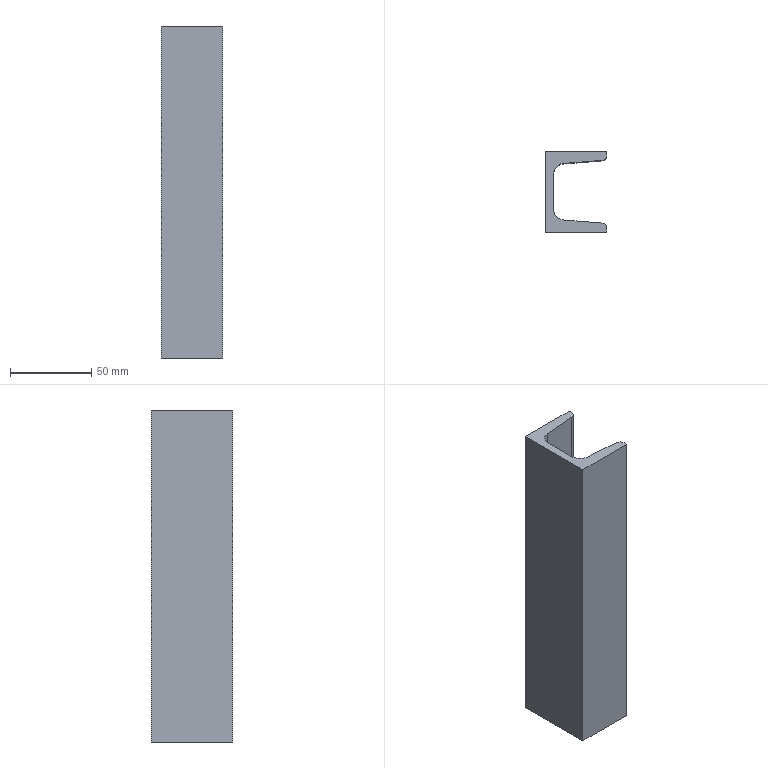Part | STEP file | DIN 1026-1 U 50 1785357045599 | 1 solid | 14 faces | box 38 x 50 x 204.153 mm | volume 145329 mm3 | plane 10 | cylinder 4 | commonest cylinder face diameters 7 x2 14 x2
STEP:
#1=CARTESIAN_POINT('',(5.,-10.418,254.153));
#2=VERTEX_POINT('',#1);
#3=CARTESIAN_POINT('',(11.442,-17.395,254.153));
#4=VERTEX_POINT('',#3);
#5=CARTESIAN_POINT('',(12.,-10.418,254.153));
#6=DIRECTION('',(0.,0.,1.));
#7=DIRECTION('',(-1.,0.,0.));
#8=AXIS2_PLACEMENT_3D('',#5,#6,#7);
#9=CIRCLE('',#8,7.);
#10=EDGE_CURVE('',#2,#4,#9,.T.);
#11=ORIENTED_EDGE('',*,*,#10,.T.);
#12=CARTESIAN_POINT('',(11.442,-17.395,50.));
#13=VERTEX_POINT('',#12);
#14=CARTESIAN_POINT('',(11.442,-17.395,0.));
#15=DIRECTION('',(0.,0.,1.));
#16=VECTOR('',#15,10.);
#17=LINE('',#14,#16);
#18=EDGE_CURVE('',#13,#4,#17,.T.);
#19=ORIENTED_EDGE('',*,*,#18,.F.);
#20=CARTESIAN_POINT('',(5.,-10.418,50.));
#21=VERTEX_POINT('',#20);
#22=CARTESIAN_POINT('',(12.,-10.418,50.));
#23=DIRECTION('',(0.,0.,1.));
#24=DIRECTION('',(-1.,0.,0.));
#25=AXIS2_PLACEMENT_3D('',#22,#23,#24);
#26=CIRCLE('',#25,7.);
#27=EDGE_CURVE('',#21,#13,#26,.T.);
#28=ORIENTED_EDGE('',*,*,#27,.F.);
#29=CARTESIAN_POINT('',(5.,-10.418,0.));
#30=DIRECTION('',(0.,0.,1.));
#31=VECTOR('',#30,10.);
#32=LINE('',#29,#31);
#33=EDGE_CURVE('',#21,#2,#32,.T.);
#34=ORIENTED_EDGE('',*,*,#33,.T.);
#35=EDGE_LOOP('',(#11,#19,#28,#34));
#36=FACE_OUTER_BOUND('',#35,.T.);
#37=CARTESIAN_POINT('',(12.,-10.418,0.));
#38=DIRECTION('',(0.,0.,1.));
#39=DIRECTION('',(-1.,0.,0.));
#40=AXIS2_PLACEMENT_3D('',#37,#38,#39);
#41=CYLINDRICAL_SURFACE('',#40,7.);
#42=ADVANCED_FACE('',(#36),#41,.F.);
#43=CARTESIAN_POINT('',(34.779,-19.262,254.153));
#44=VERTEX_POINT('',#43);
#45=CARTESIAN_POINT('',(14.505,-17.64,254.153));
#46=DIRECTION('',(0.9968,-0.07975,0.));
#47=VECTOR('',#46,10.);
#48=LINE('',#45,#47);
#49=EDGE_CURVE('',#4,#44,#48,.T.);
#50=ORIENTED_EDGE('',*,*,#49,.T.);
#51=CARTESIAN_POINT('',(34.779,-19.262,50.));
#52=VERTEX_POINT('',#51);
#53=CARTESIAN_POINT('',(34.779,-19.262,0.));
#54=DIRECTION('',(0.,0.,1.));
#55=VECTOR('',#54,10.);
#56=LINE('',#53,#55);
#57=EDGE_CURVE('',#52,#44,#56,.T.);
#58=ORIENTED_EDGE('',*,*,#57,.F.);
#59=CARTESIAN_POINT('',(14.505,-17.64,50.));
#60=DIRECTION('',(0.9968,-0.07975,0.));
#61=VECTOR('',#60,10.);
#62=LINE('',#59,#61);
#63=EDGE_CURVE('',#13,#52,#62,.T.);
#64=ORIENTED_EDGE('',*,*,#63,.F.);
#65=ORIENTED_EDGE('',*,*,#18,.T.);
#66=EDGE_LOOP('',(#50,#58,#64,#65));
#67=FACE_OUTER_BOUND('',#66,.T.);
#68=CARTESIAN_POINT('',(11.442,-17.395,0.));
#69=DIRECTION('',(0.07975,0.9968,0.));
#70=DIRECTION('',(0.,0.,1.));
#71=AXIS2_PLACEMENT_3D('',#68,#69,#70);
#72=PLANE('',#71);
#73=ADVANCED_FACE('',(#67),#72,.T.);
#74=CARTESIAN_POINT('',(38.,-22.751,254.153));
#75=VERTEX_POINT('',#74);
#76=CARTESIAN_POINT('',(34.5,-22.751,254.153));
#77=DIRECTION('',(0.,0.,-1.));
#78=DIRECTION('',(-1.,0.,0.));
#79=AXIS2_PLACEMENT_3D('',#76,#77,#78);
#80=CIRCLE('',#79,3.5);
#81=EDGE_CURVE('',#44,#75,#80,.T.);
#82=ORIENTED_EDGE('',*,*,#81,.T.);
#83=CARTESIAN_POINT('',(38.,-22.751,50.));
#84=VERTEX_POINT('',#83);
#85=CARTESIAN_POINT('',(38.,-22.751,0.));
#86=DIRECTION('',(0.,0.,1.));
#87=VECTOR('',#86,10.);
#88=LINE('',#85,#87);
#89=EDGE_CURVE('',#84,#75,#88,.T.);
#90=ORIENTED_EDGE('',*,*,#89,.F.);
#91=CARTESIAN_POINT('',(34.5,-22.751,50.));
#92=DIRECTION('',(0.,0.,-1.));
#93=DIRECTION('',(-1.,0.,0.));
#94=AXIS2_PLACEMENT_3D('',#91,#92,#93);
#95=CIRCLE('',#94,3.5);
#96=EDGE_CURVE('',#52,#84,#95,.T.);
#97=ORIENTED_EDGE('',*,*,#96,.F.);
#98=ORIENTED_EDGE('',*,*,#57,.T.);
#99=EDGE_LOOP('',(#82,#90,#97,#98));
#100=FACE_OUTER_BOUND('',#99,.T.);
#101=CARTESIAN_POINT('',(34.5,-22.751,0.));
#102=DIRECTION('',(0.,0.,1.));
#103=DIRECTION('',(-1.,0.,0.));
#104=AXIS2_PLACEMENT_3D('',#101,#102,#103);
#105=CYLINDRICAL_SURFACE('',#104,3.5);
#106=ADVANCED_FACE('',(#100),#105,.T.);
#107=CARTESIAN_POINT('',(38.,-25.,254.153));
#108=VERTEX_POINT('',#107);
#109=CARTESIAN_POINT('',(38.,-11.376,254.153));
#110=DIRECTION('',(0.,-1.,0.));
#111=VECTOR('',#110,10.);
#112=LINE('',#109,#111);
#113=EDGE_CURVE('',#75,#108,#112,.T.);
#114=ORIENTED_EDGE('',*,*,#113,.T.);
#115=CARTESIAN_POINT('',(38.,-25.,50.));
#116=VERTEX_POINT('',#115);
#117=CARTESIAN_POINT('',(38.,-25.,0.));
#118=DIRECTION('',(0.,0.,1.));
#119=VECTOR('',#118,10.);
#120=LINE('',#117,#119);
#121=EDGE_CURVE('',#116,#108,#120,.T.);
#122=ORIENTED_EDGE('',*,*,#121,.F.);
#123=CARTESIAN_POINT('',(38.,-11.376,50.));
#124=DIRECTION('',(0.,-1.,0.));
#125=VECTOR('',#124,10.);
#126=LINE('',#123,#125);
#127=EDGE_CURVE('',#84,#116,#126,.T.);
#128=ORIENTED_EDGE('',*,*,#127,.F.);
#129=ORIENTED_EDGE('',*,*,#89,.T.);
#130=EDGE_LOOP('',(#114,#122,#128,#129));
#131=FACE_OUTER_BOUND('',#130,.T.);
#132=CARTESIAN_POINT('',(38.,-22.751,0.));
#133=DIRECTION('',(1.,0.,0.));
#134=DIRECTION('',(0.,0.,-1.));
#135=AXIS2_PLACEMENT_3D('',#132,#133,#134);
#136=PLANE('',#135);
#137=ADVANCED_FACE('',(#131),#136,.T.);
#138=CARTESIAN_POINT('',(0.,-25.,254.153));
#139=VERTEX_POINT('',#138);
#140=CARTESIAN_POINT('',(28.5,-25.,254.153));
#141=DIRECTION('',(-1.,0.,0.));
#142=VECTOR('',#141,10.);
#143=LINE('',#140,#142);
#144=EDGE_CURVE('',#108,#139,#143,.T.);
#145=ORIENTED_EDGE('',*,*,#144,.T.);
#146=CARTESIAN_POINT('',(0.,-25.,50.));
#147=VERTEX_POINT('',#146);
#148=CARTESIAN_POINT('',(0.,-25.,0.));
#149=DIRECTION('',(0.,0.,1.));
#150=VECTOR('',#149,10.);
#151=LINE('',#148,#150);
#152=EDGE_CURVE('',#147,#139,#151,.T.);
#153=ORIENTED_EDGE('',*,*,#152,.F.);
#154=CARTESIAN_POINT('',(28.5,-25.,50.));
#155=DIRECTION('',(-1.,0.,0.));
#156=VECTOR('',#155,10.);
#157=LINE('',#154,#156);
#158=EDGE_CURVE('',#116,#147,#157,.T.);
#159=ORIENTED_EDGE('',*,*,#158,.F.);
#160=ORIENTED_EDGE('',*,*,#121,.T.);
#161=EDGE_LOOP('',(#145,#153,#159,#160));
#162=FACE_OUTER_BOUND('',#161,.T.);
#163=CARTESIAN_POINT('',(38.,-25.,0.));
#164=DIRECTION('',(0.,-1.,0.));
#165=DIRECTION('',(0.,0.,-1.));
#166=AXIS2_PLACEMENT_3D('',#163,#164,#165);
#167=PLANE('',#166);
#168=ADVANCED_FACE('',(#162),#167,.T.);
#169=CARTESIAN_POINT('',(0.,25.,254.153));
#170=VERTEX_POINT('',#169);
#171=CARTESIAN_POINT('',(0.,0.,254.153));
#172=DIRECTION('',(0.,1.,0.));
#173=VECTOR('',#172,10.);
#174=LINE('',#171,#173);
#175=EDGE_CURVE('',#139,#170,#174,.T.);
#176=ORIENTED_EDGE('',*,*,#175,.T.);
#177=CARTESIAN_POINT('',(0.,25.,50.));
#178=VERTEX_POINT('',#177);
#179=CARTESIAN_POINT('',(0.,25.,0.));
#180=DIRECTION('',(0.,0.,1.));
#181=VECTOR('',#180,10.);
#182=LINE('',#179,#181);
#183=EDGE_CURVE('',#178,#170,#182,.T.);
#184=ORIENTED_EDGE('',*,*,#183,.F.);
#185=CARTESIAN_POINT('',(0.,0.,50.));
#186=DIRECTION('',(0.,1.,0.));
#187=VECTOR('',#186,10.);
#188=LINE('',#185,#187);
#189=EDGE_CURVE('',#147,#178,#188,.T.);
#190=ORIENTED_EDGE('',*,*,#189,.F.);
#191=ORIENTED_EDGE('',*,*,#152,.T.);
#192=EDGE_LOOP('',(#176,#184,#190,#191));
#193=FACE_OUTER_BOUND('',#192,.T.);
#194=CARTESIAN_POINT('',(0.,0.,0.));
#195=DIRECTION('',(-1.,0.,0.));
#196=DIRECTION('',(0.,0.,1.));
#197=AXIS2_PLACEMENT_3D('',#194,#195,#196);
#198=PLANE('',#197);
#199=ADVANCED_FACE('',(#193),#198,.T.);
#200=CARTESIAN_POINT('',(38.,25.,254.153));
#201=VERTEX_POINT('',#200);
#202=CARTESIAN_POINT('',(9.5,25.,254.153));
#203=DIRECTION('',(1.,0.,0.));
#204=VECTOR('',#203,10.);
#205=LINE('',#202,#204);
#206=EDGE_CURVE('',#170,#201,#205,.T.);
#207=ORIENTED_EDGE('',*,*,#206,.T.);
#208=CARTESIAN_POINT('',(38.,25.,50.));
#209=VERTEX_POINT('',#208);
#210=CARTESIAN_POINT('',(38.,25.,0.));
#211=DIRECTION('',(0.,0.,1.));
#212=VECTOR('',#211,10.);
#213=LINE('',#210,#212);
#214=EDGE_CURVE('',#209,#201,#213,.T.);
#215=ORIENTED_EDGE('',*,*,#214,.F.);
#216=CARTESIAN_POINT('',(9.5,25.,50.));
#217=DIRECTION('',(1.,0.,0.));
#218=VECTOR('',#217,10.);
#219=LINE('',#216,#218);
#220=EDGE_CURVE('',#178,#209,#219,.T.);
#221=ORIENTED_EDGE('',*,*,#220,.F.);
#222=ORIENTED_EDGE('',*,*,#183,.T.);
#223=EDGE_LOOP('',(#207,#215,#221,#222));
#224=FACE_OUTER_BOUND('',#223,.T.);
#225=CARTESIAN_POINT('',(0.,25.,0.));
#226=DIRECTION('',(0.,1.,0.));
#227=DIRECTION('',(0.,0.,1.));
#228=AXIS2_PLACEMENT_3D('',#225,#226,#227);
#229=PLANE('',#228);
#230=ADVANCED_FACE('',(#224),#229,.T.);
#231=CARTESIAN_POINT('',(38.,22.751,254.153));
#232=VERTEX_POINT('',#231);
#233=CARTESIAN_POINT('',(38.,12.5,254.153));
#234=DIRECTION('',(0.,-1.,0.));
#235=VECTOR('',#234,10.);
#236=LINE('',#233,#235);
#237=EDGE_CURVE('',#201,#232,#236,.T.);
#238=ORIENTED_EDGE('',*,*,#237,.T.);
#239=CARTESIAN_POINT('',(38.,22.751,50.));
#240=VERTEX_POINT('',#239);
#241=CARTESIAN_POINT('',(38.,22.751,0.));
#242=DIRECTION('',(0.,0.,1.));
#243=VECTOR('',#242,10.);
#244=LINE('',#241,#243);
#245=EDGE_CURVE('',#240,#232,#244,.T.);
#246=ORIENTED_EDGE('',*,*,#245,.F.);
#247=CARTESIAN_POINT('',(38.,12.5,50.));
#248=DIRECTION('',(0.,-1.,0.));
#249=VECTOR('',#248,10.);
#250=LINE('',#247,#249);
#251=EDGE_CURVE('',#209,#240,#250,.T.);
#252=ORIENTED_EDGE('',*,*,#251,.F.);
#253=ORIENTED_EDGE('',*,*,#214,.T.);
#254=EDGE_LOOP('',(#238,#246,#252,#253));
#255=FACE_OUTER_BOUND('',#254,.T.);
#256=CARTESIAN_POINT('',(38.,25.,0.));
#257=DIRECTION('',(1.,0.,0.));
#258=DIRECTION('',(0.,0.,-1.));
#259=AXIS2_PLACEMENT_3D('',#256,#257,#258);
#260=PLANE('',#259);
#261=ADVANCED_FACE('',(#255),#260,.T.);
#262=CARTESIAN_POINT('',(34.779,19.262,254.153));
#263=VERTEX_POINT('',#262);
#264=CARTESIAN_POINT('',(34.5,22.751,254.153));
#265=DIRECTION('',(0.,0.,-1.));
#266=DIRECTION('',(-0.07975,0.9968,0.));
#267=AXIS2_PLACEMENT_3D('',#264,#265,#266);
#268=CIRCLE('',#267,3.5);
#269=EDGE_CURVE('',#232,#263,#268,.T.);
#270=ORIENTED_EDGE('',*,*,#269,.T.);
#271=CARTESIAN_POINT('',(34.779,19.262,50.));
#272=VERTEX_POINT('',#271);
#273=CARTESIAN_POINT('',(34.779,19.262,0.));
#274=DIRECTION('',(0.,0.,1.));
#275=VECTOR('',#274,10.);
#276=LINE('',#273,#275);
#277=EDGE_CURVE('',#272,#263,#276,.T.);
#278=ORIENTED_EDGE('',*,*,#277,.F.);
#279=CARTESIAN_POINT('',(34.5,22.751,50.));
#280=DIRECTION('',(0.,0.,-1.));
#281=DIRECTION('',(-0.07975,0.9968,0.));
#282=AXIS2_PLACEMENT_3D('',#279,#280,#281);
#283=CIRCLE('',#282,3.5);
#284=EDGE_CURVE('',#240,#272,#283,.T.);
#285=ORIENTED_EDGE('',*,*,#284,.F.);
#286=ORIENTED_EDGE('',*,*,#245,.T.);
#287=EDGE_LOOP('',(#270,#278,#285,#286));
#288=FACE_OUTER_BOUND('',#287,.T.);
#289=CARTESIAN_POINT('',(34.5,22.751,0.));
#290=DIRECTION('',(0.,0.,1.));
#291=DIRECTION('',(-0.07975,0.9968,0.));
#292=AXIS2_PLACEMENT_3D('',#289,#290,#291);
#293=CYLINDRICAL_SURFACE('',#292,3.5);
#294=ADVANCED_FACE('',(#288),#293,.T.);
#295=CARTESIAN_POINT('',(11.442,17.395,254.153));
#296=VERTEX_POINT('',#295);
#297=CARTESIAN_POINT('',(26.174,18.574,254.153));
#298=DIRECTION('',(-0.9968,-0.07975,0.));
#299=VECTOR('',#298,10.);
#300=LINE('',#297,#299);
#301=EDGE_CURVE('',#263,#296,#300,.T.);
#302=ORIENTED_EDGE('',*,*,#301,.T.);
#303=CARTESIAN_POINT('',(11.442,17.395,50.));
#304=VERTEX_POINT('',#303);
#305=CARTESIAN_POINT('',(11.442,17.395,0.));
#306=DIRECTION('',(0.,0.,1.));
#307=VECTOR('',#306,10.);
#308=LINE('',#305,#307);
#309=EDGE_CURVE('',#304,#296,#308,.T.);
#310=ORIENTED_EDGE('',*,*,#309,.F.);
#311=CARTESIAN_POINT('',(26.174,18.574,50.));
#312=DIRECTION('',(-0.9968,-0.07975,0.));
#313=VECTOR('',#312,10.);
#314=LINE('',#311,#313);
#315=EDGE_CURVE('',#272,#304,#314,.T.);
#316=ORIENTED_EDGE('',*,*,#315,.F.);
#317=ORIENTED_EDGE('',*,*,#277,.T.);
#318=EDGE_LOOP('',(#302,#310,#316,#317));
#319=FACE_OUTER_BOUND('',#318,.T.);
#320=CARTESIAN_POINT('',(34.779,19.262,0.));
#321=DIRECTION('',(0.07975,-0.9968,0.));
#322=DIRECTION('',(0.,0.,-1.));
#323=AXIS2_PLACEMENT_3D('',#320,#321,#322);
#324=PLANE('',#323);
#325=ADVANCED_FACE('',(#319),#324,.T.);
#326=CARTESIAN_POINT('',(5.,10.418,254.153));
#327=VERTEX_POINT('',#326);
#328=CARTESIAN_POINT('',(12.,10.418,254.153));
#329=DIRECTION('',(0.,0.,1.));
#330=DIRECTION('',(-0.07975,0.9968,0.));
#331=AXIS2_PLACEMENT_3D('',#328,#329,#330);
#332=CIRCLE('',#331,7.);
#333=EDGE_CURVE('',#296,#327,#332,.T.);
#334=ORIENTED_EDGE('',*,*,#333,.T.);
#335=CARTESIAN_POINT('',(5.,10.418,50.));
#336=VERTEX_POINT('',#335);
#337=CARTESIAN_POINT('',(5.,10.418,0.));
#338=DIRECTION('',(0.,0.,1.));
#339=VECTOR('',#338,10.);
#340=LINE('',#337,#339);
#341=EDGE_CURVE('',#336,#327,#340,.T.);
#342=ORIENTED_EDGE('',*,*,#341,.F.);
#343=CARTESIAN_POINT('',(12.,10.418,50.));
#344=DIRECTION('',(0.,0.,1.));
#345=DIRECTION('',(-0.07975,0.9968,0.));
#346=AXIS2_PLACEMENT_3D('',#343,#344,#345);
#347=CIRCLE('',#346,7.);
#348=EDGE_CURVE('',#304,#336,#347,.T.);
#349=ORIENTED_EDGE('',*,*,#348,.F.);
#350=ORIENTED_EDGE('',*,*,#309,.T.);
#351=EDGE_LOOP('',(#334,#342,#349,#350));
#352=FACE_OUTER_BOUND('',#351,.T.);
#353=CARTESIAN_POINT('',(12.,10.418,0.));
#354=DIRECTION('',(0.,0.,1.));
#355=DIRECTION('',(-0.07975,0.9968,0.));
#356=AXIS2_PLACEMENT_3D('',#353,#354,#355);
#357=CYLINDRICAL_SURFACE('',#356,7.);
#358=ADVANCED_FACE('',(#352),#357,.F.);
#359=CARTESIAN_POINT('',(5.,0.,254.153));
#360=DIRECTION('',(0.,-1.,0.));
#361=VECTOR('',#360,10.);
#362=LINE('',#359,#361);
#363=EDGE_CURVE('',#327,#2,#362,.T.);
#364=ORIENTED_EDGE('',*,*,#363,.T.);
#365=ORIENTED_EDGE('',*,*,#33,.F.);
#366=CARTESIAN_POINT('',(5.,0.,50.));
#367=DIRECTION('',(0.,-1.,0.));
#368=VECTOR('',#367,10.);
#369=LINE('',#366,#368);
#370=EDGE_CURVE('',#336,#21,#369,.T.);
#371=ORIENTED_EDGE('',*,*,#370,.F.);
#372=ORIENTED_EDGE('',*,*,#341,.T.);
#373=EDGE_LOOP('',(#364,#365,#371,#372));
#374=FACE_OUTER_BOUND('',#373,.T.);
#375=CARTESIAN_POINT('',(5.,0.,0.));
#376=DIRECTION('',(1.,0.,0.));
#377=DIRECTION('',(0.,0.,-1.));
#378=AXIS2_PLACEMENT_3D('',#375,#376,#377);
#379=PLANE('',#378);
#380=ADVANCED_FACE('',(#374),#379,.T.);
#381=ORIENTED_EDGE('',*,*,#220,.T.);
#382=ORIENTED_EDGE('',*,*,#251,.T.);
#383=ORIENTED_EDGE('',*,*,#284,.T.);
#384=ORIENTED_EDGE('',*,*,#315,.T.);
#385=ORIENTED_EDGE('',*,*,#348,.T.);
#386=ORIENTED_EDGE('',*,*,#370,.T.);
#387=ORIENTED_EDGE('',*,*,#27,.T.);
#388=ORIENTED_EDGE('',*,*,#63,.T.);
#389=ORIENTED_EDGE('',*,*,#96,.T.);
#390=ORIENTED_EDGE('',*,*,#127,.T.);
#391=ORIENTED_EDGE('',*,*,#158,.T.);
#392=ORIENTED_EDGE('',*,*,#189,.T.);
#393=EDGE_LOOP('',(#381,#382,#383,#384,#385,#386,#387,#388,#389,#390,#391,#392));
#394=FACE_OUTER_BOUND('',#393,.T.);
#395=CARTESIAN_POINT('',(19.,0.,50.));
#396=DIRECTION('',(0.,0.,1.));
#397=DIRECTION('',(1.,0.,0.));
#398=AXIS2_PLACEMENT_3D('',#395,#396,#397);
#399=PLANE('',#398);
#400=ADVANCED_FACE('',(#394),#399,.F.);
#401=ORIENTED_EDGE('',*,*,#206,.F.);
#402=ORIENTED_EDGE('',*,*,#175,.F.);
#403=ORIENTED_EDGE('',*,*,#144,.F.);
#404=ORIENTED_EDGE('',*,*,#113,.F.);
#405=ORIENTED_EDGE('',*,*,#81,.F.);
#406=ORIENTED_EDGE('',*,*,#49,.F.);
#407=ORIENTED_EDGE('',*,*,#10,.F.);
#408=ORIENTED_EDGE('',*,*,#363,.F.);
#409=ORIENTED_EDGE('',*,*,#333,.F.);
#410=ORIENTED_EDGE('',*,*,#301,.F.);
#411=ORIENTED_EDGE('',*,*,#269,.F.);
#412=ORIENTED_EDGE('',*,*,#237,.F.);
#413=EDGE_LOOP('',(#401,#402,#403,#404,#405,#406,#407,#408,#409,#410,#411,#412));
#414=FACE_OUTER_BOUND('',#413,.T.);
#415=CARTESIAN_POINT('',(19.,0.,254.153));
#416=DIRECTION('',(0.,0.,1.));
#417=DIRECTION('',(1.,0.,0.));
#418=AXIS2_PLACEMENT_3D('',#415,#416,#417);
#419=PLANE('',#418);
#420=ADVANCED_FACE('',(#414),#419,.T.);
#421=CLOSED_SHELL('',(#42,#73,#106,#137,#168,#199,#230,#261,#294,#325,#358,#380,#400,#420));
#422=MANIFOLD_SOLID_BREP('',#421);
#423=(LENGTH_UNIT()NAMED_UNIT(*)SI_UNIT(.MILLI.,.METRE.));
#424=UNCERTAINTY_MEASURE_WITH_UNIT(LENGTH_MEASURE(0.01),#423,'','');
#425=(NAMED_UNIT(*)PLANE_ANGLE_UNIT()SI_UNIT($,.RADIAN.));
#426=(NAMED_UNIT(*)SI_UNIT($,.STERADIAN.)SOLID_ANGLE_UNIT());
#427=(GEOMETRIC_REPRESENTATION_CONTEXT(3)GLOBAL_UNCERTAINTY_ASSIGNED_CONTEXT((#424))GLOBAL_UNIT_ASSIGNED_CONTEXT((#423,#425,#426))REPRESENTATION_CONTEXT('',''));
#428=ADVANCED_BREP_SHAPE_REPRESENTATION('',(#422),#427);